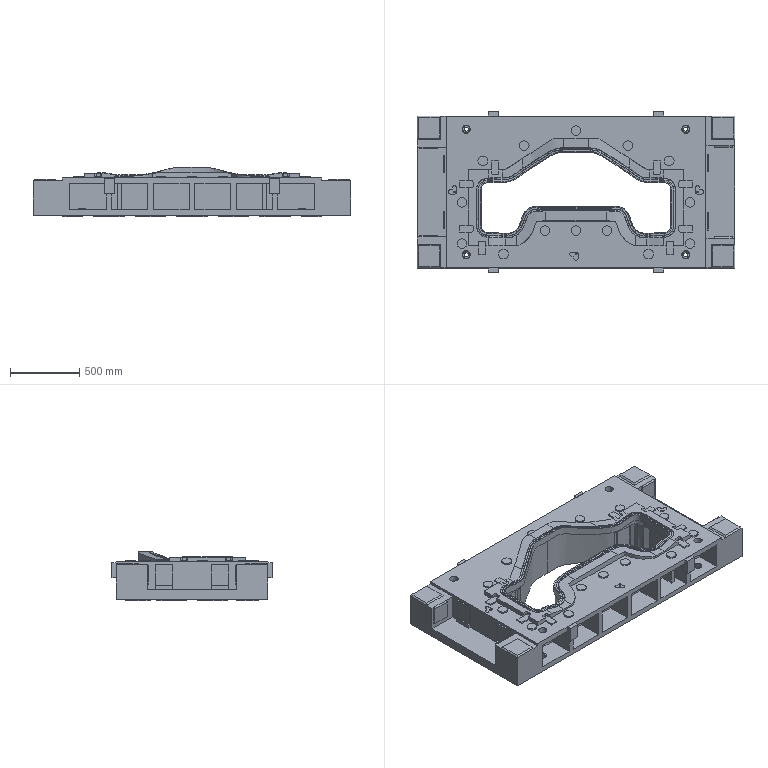Part | NX | features solid 2 | 1 solid | 793 faces | box 2300 x 1160 x 356.885 mm | volume 290684414 mm3 | plane 547 | cylinder 140 | spline 103 | cone 3 | commonest cylinder face diameters 70 x58 20 x34 16 x17 30 x13 10 x6 40 x4